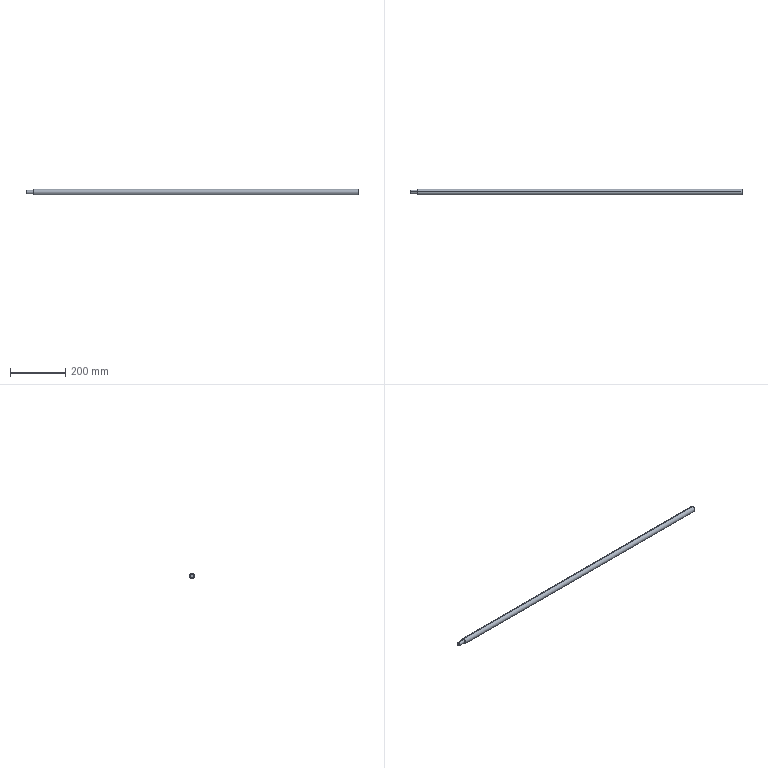Part | STEP file | 1 solid | 7 faces | box 1200 x 20 x 20 mm | volume 371431 mm3 | cylinder 4 | plane 3 | commonest cylinder face diameters 12.131 x2 20 x2
STEP:
#1=CARTESIAN_POINT('',(0.,0.,0.));
#2=DIRECTION('',(0.,0.,1.));
#3=DIRECTION('',(1.,0.,0.));
#4=AXIS2_PLACEMENT_3D('',#1,#2,#3);
#5=CARTESIAN_POINT('',(-572.,553.5,110.971));
#6=VERTEX_POINT('',#5);
#7=CARTESIAN_POINT('',(-572.,553.5,98.84));
#8=VERTEX_POINT('',#7);
#9=CARTESIAN_POINT('',(-572.,553.5,104.906));
#10=DIRECTION('',(-1.,0.,0.));
#11=DIRECTION('',(0.,0.,1.));
#12=AXIS2_PLACEMENT_3D('',#9,#10,#11);
#13=CIRCLE('',#12,6.065);
#14=CARTESIAN_POINT('',(-572.,553.5,104.906));
#15=DIRECTION('',(-1.,0.,0.));
#16=DIRECTION('',(0.,0.,1.));
#17=AXIS2_PLACEMENT_3D('',#14,#15,#16);
#18=CYLINDRICAL_SURFACE('',#17,6.065);
#19=CARTESIAN_POINT('',(0.,0.));
#20=DIRECTION('',(1.,0.));
#21=VECTOR('',#20,1.);
#22=LINE('',#19,#21);
#23=(GEOMETRIC_REPRESENTATION_CONTEXT(2)PARAMETRIC_REPRESENTATION_CONTEXT()REPRESENTATION_CONTEXT('',''));
#24=DEFINITIONAL_REPRESENTATION('',(#22),#23);
#25=PCURVE('',#18,#24);
#26=CARTESIAN_POINT('',(-572.,553.5,104.906));
#27=DIRECTION('',(-1.,0.,0.));
#28=DIRECTION('',(0.,0.,1.));
#29=AXIS2_PLACEMENT_3D('',#26,#27,#28);
#30=PLANE('',#29);
#31=CARTESIAN_POINT('',(0.,0.));
#32=DIRECTION('',(1.,0.));
#33=AXIS2_PLACEMENT_2D('',#31,#32);
#34=CIRCLE('',#33,6.065);
#35=(GEOMETRIC_REPRESENTATION_CONTEXT(2)PARAMETRIC_REPRESENTATION_CONTEXT()REPRESENTATION_CONTEXT('',''));
#36=DEFINITIONAL_REPRESENTATION('',(#34),#35);
#37=PCURVE('',#30,#36);
#38=SURFACE_CURVE('',#13,(#25,#37),.PCURVE_S1.);
#39=EDGE_CURVE('',#6,#8,#38,.T.);
#40=ORIENTED_EDGE('',*,*,#39,.T.);
#41=CARTESIAN_POINT('',(-600.,553.5,98.84));
#42=VERTEX_POINT('',#41);
#43=CARTESIAN_POINT('',(-572.,553.5,98.84));
#44=DIRECTION('',(-1.,0.,0.));
#45=VECTOR('',#44,1.);
#46=LINE('',#43,#45);
#47=CARTESIAN_POINT('',(3.142,0.));
#48=DIRECTION('',(0.,1.));
#49=VECTOR('',#48,1.);
#50=LINE('',#47,#49);
#51=(GEOMETRIC_REPRESENTATION_CONTEXT(2)PARAMETRIC_REPRESENTATION_CONTEXT()REPRESENTATION_CONTEXT('',''));
#52=DEFINITIONAL_REPRESENTATION('',(#50),#51);
#53=PCURVE('',#18,#52);
#54=CARTESIAN_POINT('',(-572.,553.5,104.906));
#55=DIRECTION('',(-1.,0.,0.));
#56=DIRECTION('',(0.,0.,1.));
#57=AXIS2_PLACEMENT_3D('',#54,#55,#56);
#58=CYLINDRICAL_SURFACE('',#57,6.065);
#59=CARTESIAN_POINT('',(3.142,0.));
#60=DIRECTION('',(0.,1.));
#61=VECTOR('',#60,1.);
#62=LINE('',#59,#61);
#63=(GEOMETRIC_REPRESENTATION_CONTEXT(2)PARAMETRIC_REPRESENTATION_CONTEXT()REPRESENTATION_CONTEXT('',''));
#64=DEFINITIONAL_REPRESENTATION('',(#62),#63);
#65=PCURVE('',#58,#64);
#66=SURFACE_CURVE('',#46,(#53,#65),.PCURVE_S1.);
#67=EDGE_CURVE('',#8,#42,#66,.T.);
#68=ORIENTED_EDGE('',*,*,#67,.T.);
#69=CARTESIAN_POINT('',(-600.,553.5,110.971));
#70=VERTEX_POINT('',#69);
#71=CARTESIAN_POINT('',(-600.,553.5,104.906));
#72=DIRECTION('',(-1.,0.,0.));
#73=DIRECTION('',(0.,0.,1.));
#74=AXIS2_PLACEMENT_3D('',#71,#72,#73);
#75=CIRCLE('',#74,6.065);
#76=CARTESIAN_POINT('',(0.,28.));
#77=DIRECTION('',(1.,0.));
#78=VECTOR('',#77,1.);
#79=LINE('',#76,#78);
#80=(GEOMETRIC_REPRESENTATION_CONTEXT(2)PARAMETRIC_REPRESENTATION_CONTEXT()REPRESENTATION_CONTEXT('',''));
#81=DEFINITIONAL_REPRESENTATION('',(#79),#80);
#82=PCURVE('',#18,#81);
#83=CARTESIAN_POINT('',(-600.,553.5,104.906));
#84=DIRECTION('',(-1.,0.,0.));
#85=DIRECTION('',(0.,0.,1.));
#86=AXIS2_PLACEMENT_3D('',#83,#84,#85);
#87=PLANE('',#86);
#88=CARTESIAN_POINT('',(0.,0.));
#89=DIRECTION('',(1.,0.));
#90=AXIS2_PLACEMENT_2D('',#88,#89);
#91=CIRCLE('',#90,6.065);
#92=(GEOMETRIC_REPRESENTATION_CONTEXT(2)PARAMETRIC_REPRESENTATION_CONTEXT()REPRESENTATION_CONTEXT('',''));
#93=DEFINITIONAL_REPRESENTATION('',(#91),#92);
#94=PCURVE('',#87,#93);
#95=SURFACE_CURVE('',#75,(#82,#94),.PCURVE_S1.);
#96=EDGE_CURVE('',#70,#42,#95,.T.);
#97=ORIENTED_EDGE('',*,*,#96,.F.);
#98=CARTESIAN_POINT('',(-572.,553.5,110.971));
#99=DIRECTION('',(-1.,0.,0.));
#100=VECTOR('',#99,1.);
#101=LINE('',#98,#100);
#102=CARTESIAN_POINT('',(0.,0.));
#103=DIRECTION('',(0.,1.));
#104=VECTOR('',#103,1.);
#105=LINE('',#102,#104);
#106=(GEOMETRIC_REPRESENTATION_CONTEXT(2)PARAMETRIC_REPRESENTATION_CONTEXT()REPRESENTATION_CONTEXT('',''));
#107=DEFINITIONAL_REPRESENTATION('',(#105),#106);
#108=PCURVE('',#18,#107);
#109=CARTESIAN_POINT('',(6.283,0.));
#110=DIRECTION('',(0.,1.));
#111=VECTOR('',#110,1.);
#112=LINE('',#109,#111);
#113=(GEOMETRIC_REPRESENTATION_CONTEXT(2)PARAMETRIC_REPRESENTATION_CONTEXT()REPRESENTATION_CONTEXT('',''));
#114=DEFINITIONAL_REPRESENTATION('',(#112),#113);
#115=PCURVE('',#58,#114);
#116=SURFACE_CURVE('',#101,(#108,#115),.PCURVE_S1.);
#117=EDGE_CURVE('',#6,#70,#116,.T.);
#118=ORIENTED_EDGE('',*,*,#117,.F.);
#119=EDGE_LOOP('',(#40,#68,#97,#118));
#120=FACE_BOUND('',#119,.T.);
#121=ADVANCED_FACE('',(#120),#18,.T.);
#122=CARTESIAN_POINT('',(600.,553.5,114.906));
#123=VERTEX_POINT('',#122);
#124=CARTESIAN_POINT('',(600.,553.5,94.906));
#125=VERTEX_POINT('',#124);
#126=CARTESIAN_POINT('',(600.,553.5,104.906));
#127=DIRECTION('',(-1.,0.,0.));
#128=DIRECTION('',(0.,0.,-1.));
#129=AXIS2_PLACEMENT_3D('',#126,#127,#128);
#130=CIRCLE('',#129,10.);
#131=CARTESIAN_POINT('',(628.284,553.5,104.906));
#132=DIRECTION('',(-1.,0.,0.));
#133=DIRECTION('',(0.,0.,1.));
#134=AXIS2_PLACEMENT_3D('',#131,#132,#133);
#135=CYLINDRICAL_SURFACE('',#134,10.);
#136=CARTESIAN_POINT('',(-3.142,28.284));
#137=DIRECTION('',(1.,0.));
#138=VECTOR('',#137,1.);
#139=LINE('',#136,#138);
#140=(GEOMETRIC_REPRESENTATION_CONTEXT(2)PARAMETRIC_REPRESENTATION_CONTEXT()REPRESENTATION_CONTEXT('',''));
#141=DEFINITIONAL_REPRESENTATION('',(#139),#140);
#142=PCURVE('',#135,#141);
#143=CARTESIAN_POINT('',(600.,454.347,-79.086));
#144=DIRECTION('',(1.,0.,0.));
#145=DIRECTION('',(0.,0.,-1.));
#146=AXIS2_PLACEMENT_3D('',#143,#144,#145);
#147=PLANE('',#146);
#148=CARTESIAN_POINT('',(-173.991,99.153));
#149=CARTESIAN_POINT('',(-173.991,81.833));
#150=CARTESIAN_POINT('',(-188.991,90.493));
#151=CARTESIAN_POINT('',(-203.991,99.153));
#152=CARTESIAN_POINT('',(-188.991,107.814));
#153=CARTESIAN_POINT('',(-173.991,116.474));
#154=CARTESIAN_POINT('',(-173.991,99.153));
#155=(BOUNDED_CURVE()B_SPLINE_CURVE(2,(#148,#149,#150,#151,#152,#153,#154),.UNSPECIFIED.,.T.,.F.)B_SPLINE_CURVE_WITH_KNOTS((1,2,2,2,2,1),(-2.094,0.,2.094,4.189,6.283,8.378),.UNSPECIFIED.)CURVE()GEOMETRIC_REPRESENTATION_ITEM()RATIONAL_B_SPLINE_CURVE((1.,0.5,1.,0.5,1.,0.5,1.))REPRESENTATION_ITEM(''));
#156=(GEOMETRIC_REPRESENTATION_CONTEXT(2)PARAMETRIC_REPRESENTATION_CONTEXT()REPRESENTATION_CONTEXT('',''));
#157=DEFINITIONAL_REPRESENTATION('',(#155),#156);
#158=PCURVE('',#147,#157);
#159=SURFACE_CURVE('',#130,(#142,#158),.PCURVE_S1.);
#160=EDGE_CURVE('',#123,#125,#159,.T.);
#161=ORIENTED_EDGE('',*,*,#160,.T.);
#162=CARTESIAN_POINT('',(-572.,553.5,94.906));
#163=VERTEX_POINT('',#162);
#164=CARTESIAN_POINT('',(628.284,553.5,94.906));
#165=DIRECTION('',(-1.,0.,0.));
#166=VECTOR('',#165,1.);
#167=LINE('',#164,#166);
#168=CARTESIAN_POINT('',(3.142,0.));
#169=DIRECTION('',(0.,1.));
#170=VECTOR('',#169,1.);
#171=LINE('',#168,#170);
#172=(GEOMETRIC_REPRESENTATION_CONTEXT(2)PARAMETRIC_REPRESENTATION_CONTEXT()REPRESENTATION_CONTEXT('',''));
#173=DEFINITIONAL_REPRESENTATION('',(#171),#172);
#174=PCURVE('',#135,#173);
#175=CARTESIAN_POINT('',(628.284,553.5,104.906));
#176=DIRECTION('',(-1.,0.,0.));
#177=DIRECTION('',(0.,0.,1.));
#178=AXIS2_PLACEMENT_3D('',#175,#176,#177);
#179=CYLINDRICAL_SURFACE('',#178,10.);
#180=CARTESIAN_POINT('',(3.142,0.));
#181=DIRECTION('',(0.,1.));
#182=VECTOR('',#181,1.);
#183=LINE('',#180,#182);
#184=(GEOMETRIC_REPRESENTATION_CONTEXT(2)PARAMETRIC_REPRESENTATION_CONTEXT()REPRESENTATION_CONTEXT('',''));
#185=DEFINITIONAL_REPRESENTATION('',(#183),#184);
#186=PCURVE('',#179,#185);
#187=SURFACE_CURVE('',#167,(#174,#186),.PCURVE_S1.);
#188=EDGE_CURVE('',#125,#163,#187,.T.);
#189=ORIENTED_EDGE('',*,*,#188,.T.);
#190=CARTESIAN_POINT('',(-572.,553.5,114.906));
#191=VERTEX_POINT('',#190);
#192=CARTESIAN_POINT('',(-572.,553.5,104.906));
#193=DIRECTION('',(1.,0.,0.));
#194=DIRECTION('',(0.,0.,1.));
#195=AXIS2_PLACEMENT_3D('',#192,#193,#194);
#196=CIRCLE('',#195,10.);
#197=CARTESIAN_POINT('',(6.283,1200.284));
#198=DIRECTION('',(-1.,0.));
#199=VECTOR('',#198,1.);
#200=LINE('',#197,#199);
#201=(GEOMETRIC_REPRESENTATION_CONTEXT(2)PARAMETRIC_REPRESENTATION_CONTEXT()REPRESENTATION_CONTEXT('',''));
#202=DEFINITIONAL_REPRESENTATION('',(#200),#201);
#203=PCURVE('',#135,#202);
#204=CARTESIAN_POINT('',(10.,0.));
#205=CARTESIAN_POINT('',(10.,-17.321));
#206=CARTESIAN_POINT('',(-5.,-8.66));
#207=CARTESIAN_POINT('',(-20.,0.));
#208=CARTESIAN_POINT('',(-5.,8.66));
#209=CARTESIAN_POINT('',(10.,17.321));
#210=CARTESIAN_POINT('',(10.,0.));
#211=(BOUNDED_CURVE()B_SPLINE_CURVE(2,(#204,#205,#206,#207,#208,#209,#210),.UNSPECIFIED.,.T.,.F.)B_SPLINE_CURVE_WITH_KNOTS((1,2,2,2,2,1),(-2.094,0.,2.094,4.189,6.283,8.378),.UNSPECIFIED.)CURVE()GEOMETRIC_REPRESENTATION_ITEM()RATIONAL_B_SPLINE_CURVE((1.,0.5,1.,0.5,1.,0.5,1.))REPRESENTATION_ITEM(''));
#212=(GEOMETRIC_REPRESENTATION_CONTEXT(2)PARAMETRIC_REPRESENTATION_CONTEXT()REPRESENTATION_CONTEXT('',''));
#213=DEFINITIONAL_REPRESENTATION('',(#211),#212);
#214=PCURVE('',#30,#213);
#215=SURFACE_CURVE('',#196,(#203,#214),.PCURVE_S1.);
#216=EDGE_CURVE('',#163,#191,#215,.T.);
#217=ORIENTED_EDGE('',*,*,#216,.T.);
#218=CARTESIAN_POINT('',(628.284,553.5,114.906));
#219=DIRECTION('',(-1.,0.,0.));
#220=VECTOR('',#219,1.);
#221=LINE('',#218,#220);
#222=CARTESIAN_POINT('',(0.,0.));
#223=DIRECTION('',(0.,1.));
#224=VECTOR('',#223,1.);
#225=LINE('',#222,#224);
#226=(GEOMETRIC_REPRESENTATION_CONTEXT(2)PARAMETRIC_REPRESENTATION_CONTEXT()REPRESENTATION_CONTEXT('',''));
#227=DEFINITIONAL_REPRESENTATION('',(#225),#226);
#228=PCURVE('',#135,#227);
#229=CARTESIAN_POINT('',(6.283,0.));
#230=DIRECTION('',(0.,1.));
#231=VECTOR('',#230,1.);
#232=LINE('',#229,#231);
#233=(GEOMETRIC_REPRESENTATION_CONTEXT(2)PARAMETRIC_REPRESENTATION_CONTEXT()REPRESENTATION_CONTEXT('',''));
#234=DEFINITIONAL_REPRESENTATION('',(#232),#233);
#235=PCURVE('',#179,#234);
#236=SURFACE_CURVE('',#221,(#228,#235),.PCURVE_S1.);
#237=EDGE_CURVE('',#123,#191,#236,.T.);
#238=ORIENTED_EDGE('',*,*,#237,.F.);
#239=EDGE_LOOP('',(#161,#189,#217,#238));
#240=FACE_BOUND('',#239,.T.);
#241=ADVANCED_FACE('',(#240),#135,.T.);
#242=ORIENTED_EDGE('',*,*,#188,.F.);
#243=CARTESIAN_POINT('',(600.,553.5,104.906));
#244=DIRECTION('',(-1.,0.,0.));
#245=DIRECTION('',(0.,0.,-1.));
#246=AXIS2_PLACEMENT_3D('',#243,#244,#245);
#247=CIRCLE('',#246,10.);
#248=CARTESIAN_POINT('',(3.142,28.284));
#249=DIRECTION('',(1.,0.));
#250=VECTOR('',#249,1.);
#251=LINE('',#248,#250);
#252=(GEOMETRIC_REPRESENTATION_CONTEXT(2)PARAMETRIC_REPRESENTATION_CONTEXT()REPRESENTATION_CONTEXT('',''));
#253=DEFINITIONAL_REPRESENTATION('',(#251),#252);
#254=PCURVE('',#179,#253);
#255=CARTESIAN_POINT('',(-173.991,99.153));
#256=CARTESIAN_POINT('',(-173.991,81.833));
#257=CARTESIAN_POINT('',(-188.991,90.493));
#258=CARTESIAN_POINT('',(-203.991,99.153));
#259=CARTESIAN_POINT('',(-188.991,107.814));
#260=CARTESIAN_POINT('',(-173.991,116.474));
#261=CARTESIAN_POINT('',(-173.991,99.153));
#262=(BOUNDED_CURVE()B_SPLINE_CURVE(2,(#255,#256,#257,#258,#259,#260,#261),.UNSPECIFIED.,.T.,.F.)B_SPLINE_CURVE_WITH_KNOTS((1,2,2,2,2,1),(-2.094,0.,2.094,4.189,6.283,8.378),.UNSPECIFIED.)CURVE()GEOMETRIC_REPRESENTATION_ITEM()RATIONAL_B_SPLINE_CURVE((1.,0.5,1.,0.5,1.,0.5,1.))REPRESENTATION_ITEM(''));
#263=(GEOMETRIC_REPRESENTATION_CONTEXT(2)PARAMETRIC_REPRESENTATION_CONTEXT()REPRESENTATION_CONTEXT('',''));
#264=DEFINITIONAL_REPRESENTATION('',(#262),#263);
#265=PCURVE('',#147,#264);
#266=SURFACE_CURVE('',#247,(#254,#265),.PCURVE_S1.);
#267=EDGE_CURVE('',#125,#123,#266,.T.);
#268=ORIENTED_EDGE('',*,*,#267,.T.);
#269=ORIENTED_EDGE('',*,*,#237,.T.);
#270=CARTESIAN_POINT('',(-572.,553.5,104.906));
#271=DIRECTION('',(1.,0.,0.));
#272=DIRECTION('',(0.,0.,1.));
#273=AXIS2_PLACEMENT_3D('',#270,#271,#272);
#274=CIRCLE('',#273,10.);
#275=CARTESIAN_POINT('',(6.283,1200.284));
#276=DIRECTION('',(-1.,0.));
#277=VECTOR('',#276,1.);
#278=LINE('',#275,#277);
#279=(GEOMETRIC_REPRESENTATION_CONTEXT(2)PARAMETRIC_REPRESENTATION_CONTEXT()REPRESENTATION_CONTEXT('',''));
#280=DEFINITIONAL_REPRESENTATION('',(#278),#279);
#281=PCURVE('',#179,#280);
#282=CARTESIAN_POINT('',(10.,0.));
#283=CARTESIAN_POINT('',(10.,-17.321));
#284=CARTESIAN_POINT('',(-5.,-8.66));
#285=CARTESIAN_POINT('',(-20.,0.));
#286=CARTESIAN_POINT('',(-5.,8.66));
#287=CARTESIAN_POINT('',(10.,17.321));
#288=CARTESIAN_POINT('',(10.,0.));
#289=(BOUNDED_CURVE()B_SPLINE_CURVE(2,(#282,#283,#284,#285,#286,#287,#288),.UNSPECIFIED.,.T.,.F.)B_SPLINE_CURVE_WITH_KNOTS((1,2,2,2,2,1),(-2.094,0.,2.094,4.189,6.283,8.378),.UNSPECIFIED.)CURVE()GEOMETRIC_REPRESENTATION_ITEM()RATIONAL_B_SPLINE_CURVE((1.,0.5,1.,0.5,1.,0.5,1.))REPRESENTATION_ITEM(''));
#290=(GEOMETRIC_REPRESENTATION_CONTEXT(2)PARAMETRIC_REPRESENTATION_CONTEXT()REPRESENTATION_CONTEXT('',''));
#291=DEFINITIONAL_REPRESENTATION('',(#289),#290);
#292=PCURVE('',#30,#291);
#293=SURFACE_CURVE('',#274,(#281,#292),.PCURVE_S1.);
#294=EDGE_CURVE('',#191,#163,#293,.T.);
#295=ORIENTED_EDGE('',*,*,#294,.T.);
#296=EDGE_LOOP('',(#242,#268,#269,#295));
#297=FACE_BOUND('',#296,.T.);
#298=ADVANCED_FACE('',(#297),#179,.T.);
#299=ORIENTED_EDGE('',*,*,#160,.F.);
#300=ORIENTED_EDGE('',*,*,#267,.F.);
#301=EDGE_LOOP('',(#299,#300));
#302=FACE_BOUND('',#301,.T.);
#303=ADVANCED_FACE('',(#302),#147,.T.);
#304=ORIENTED_EDGE('',*,*,#294,.F.);
#305=ORIENTED_EDGE('',*,*,#216,.F.);
#306=EDGE_LOOP('',(#304,#305));
#307=FACE_BOUND('',#306,.T.);
#308=ORIENTED_EDGE('',*,*,#39,.F.);
#309=CARTESIAN_POINT('',(-572.,553.5,104.906));
#310=DIRECTION('',(-1.,0.,0.));
#311=DIRECTION('',(0.,0.,1.));
#312=AXIS2_PLACEMENT_3D('',#309,#310,#311);
#313=CIRCLE('',#312,6.065);
#314=CARTESIAN_POINT('',(0.,0.));
#315=DIRECTION('',(1.,0.));
#316=AXIS2_PLACEMENT_2D('',#314,#315);
#317=CIRCLE('',#316,6.065);
#318=(GEOMETRIC_REPRESENTATION_CONTEXT(2)PARAMETRIC_REPRESENTATION_CONTEXT()REPRESENTATION_CONTEXT('',''));
#319=DEFINITIONAL_REPRESENTATION('',(#317),#318);
#320=PCURVE('',#30,#319);
#321=CARTESIAN_POINT('',(0.,0.));
#322=DIRECTION('',(1.,0.));
#323=VECTOR('',#322,1.);
#324=LINE('',#321,#323);
#325=(GEOMETRIC_REPRESENTATION_CONTEXT(2)PARAMETRIC_REPRESENTATION_CONTEXT()REPRESENTATION_CONTEXT('',''));
#326=DEFINITIONAL_REPRESENTATION('',(#324),#325);
#327=PCURVE('',#58,#326);
#328=SURFACE_CURVE('',#313,(#320,#327),.PCURVE_S1.);
#329=EDGE_CURVE('',#8,#6,#328,.T.);
#330=ORIENTED_EDGE('',*,*,#329,.F.);
#331=EDGE_LOOP('',(#308,#330));
#332=FACE_BOUND('',#331,.T.);
#333=ADVANCED_FACE('',(#307,#332),#30,.T.);
#334=ORIENTED_EDGE('',*,*,#67,.F.);
#335=ORIENTED_EDGE('',*,*,#329,.T.);
#336=ORIENTED_EDGE('',*,*,#117,.T.);
#337=CARTESIAN_POINT('',(-600.,553.5,104.906));
#338=DIRECTION('',(-1.,0.,0.));
#339=DIRECTION('',(0.,0.,1.));
#340=AXIS2_PLACEMENT_3D('',#337,#338,#339);
#341=CIRCLE('',#340,6.065);
#342=CARTESIAN_POINT('',(0.,28.));
#343=DIRECTION('',(1.,0.));
#344=VECTOR('',#343,1.);
#345=LINE('',#342,#344);
#346=(GEOMETRIC_REPRESENTATION_CONTEXT(2)PARAMETRIC_REPRESENTATION_CONTEXT()REPRESENTATION_CONTEXT('',''));
#347=DEFINITIONAL_REPRESENTATION('',(#345),#346);
#348=PCURVE('',#58,#347);
#349=CARTESIAN_POINT('',(0.,0.));
#350=DIRECTION('',(1.,0.));
#351=AXIS2_PLACEMENT_2D('',#349,#350);
#352=CIRCLE('',#351,6.065);
#353=(GEOMETRIC_REPRESENTATION_CONTEXT(2)PARAMETRIC_REPRESENTATION_CONTEXT()REPRESENTATION_CONTEXT('',''));
#354=DEFINITIONAL_REPRESENTATION('',(#352),#353);
#355=PCURVE('',#87,#354);
#356=SURFACE_CURVE('',#341,(#348,#355),.PCURVE_S1.);
#357=EDGE_CURVE('',#42,#70,#356,.T.);
#358=ORIENTED_EDGE('',*,*,#357,.F.);
#359=EDGE_LOOP('',(#334,#335,#336,#358));
#360=FACE_BOUND('',#359,.T.);
#361=ADVANCED_FACE('',(#360),#58,.T.);
#362=ORIENTED_EDGE('',*,*,#96,.T.);
#363=ORIENTED_EDGE('',*,*,#357,.T.);
#364=EDGE_LOOP('',(#362,#363));
#365=FACE_BOUND('',#364,.T.);
#366=ADVANCED_FACE('',(#365),#87,.T.);
#367=CLOSED_SHELL('',(#121,#241,#298,#303,#333,#361,#366));
#368=MANIFOLD_SOLID_BREP('',#367);
#369=(LENGTH_UNIT()NAMED_UNIT(*)SI_UNIT(.MILLI.,.METRE.));
#370=UNCERTAINTY_MEASURE_WITH_UNIT(LENGTH_MEASURE(0.0000001),#369,'','');
#371=(NAMED_UNIT(*)PLANE_ANGLE_UNIT()SI_UNIT($,.RADIAN.));
#372=(NAMED_UNIT(*)SI_UNIT($,.STERADIAN.)SOLID_ANGLE_UNIT());
#373=(GEOMETRIC_REPRESENTATION_CONTEXT(3)GLOBAL_UNCERTAINTY_ASSIGNED_CONTEXT((#370))GLOBAL_UNIT_ASSIGNED_CONTEXT((#369,#371,#372))REPRESENTATION_CONTEXT('',''));
#374=ADVANCED_BREP_SHAPE_REPRESENTATION('',(#4,#368),#373);